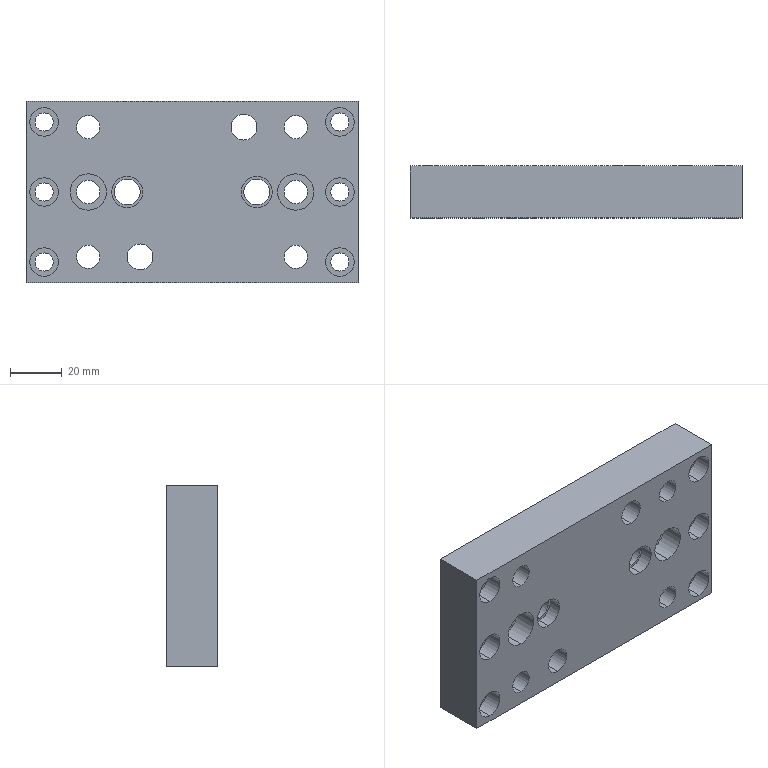Part | STEP file | OP10-130_cylinder base (2)-L | 1 solid | 74 faces | box 128 x 20 x 70 mm | volume 155973 mm3 | cylinder 56 | plane 18 | commonest cylinder face diameters 7 x12 9 x12 11 x12 10 x8 12 x8 14 x4